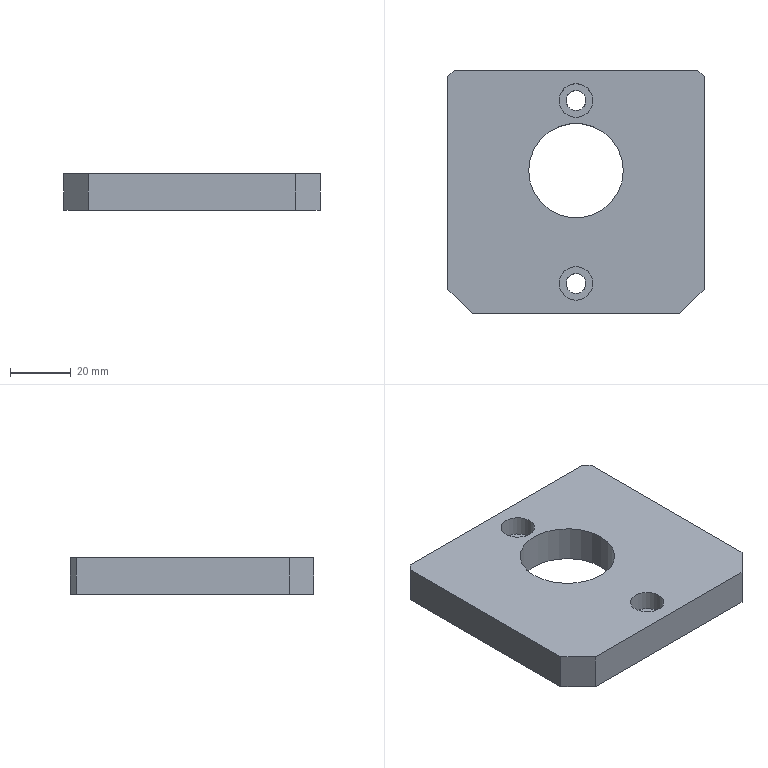Part | STEP file | P011002NM01-000 | 1 solid | 17 faces | box 84 x 80 x 12 mm | volume 69166 mm3 | plane 12 | cylinder 5 | commonest cylinder face diameters 6.5 x2 11 x2 31 x1
STEP:
#1=CARTESIAN_POINT('',(0.,0.,0.));
#2=DIRECTION('',(0.,0.,1.));
#3=DIRECTION('',(1.,0.,0.));
#4=AXIS2_PLACEMENT_3D('',#1,#2,#3);
#5=CARTESIAN_POINT('',(-104.,245.,9.));
#6=VERTEX_POINT('',#5);
#7=CARTESIAN_POINT('',(-172.,245.,9.));
#8=VERTEX_POINT('',#7);
#9=CARTESIAN_POINT('',(-140.,245.,9.));
#10=DIRECTION('',(-1.,0.,0.));
#11=VECTOR('',#10,1.);
#12=LINE('',#9,#11);
#13=CARTESIAN_POINT('',(-140.,245.,6.));
#14=DIRECTION('',(0.,-1.,0.));
#15=DIRECTION('',(0.,0.,-1.));
#16=AXIS2_PLACEMENT_3D('',#13,#14,#15);
#17=PLANE('',#16);
#18=CARTESIAN_POINT('',(-3.,0.));
#19=DIRECTION('',(0.,-1.));
#20=VECTOR('',#19,1.);
#21=LINE('',#18,#20);
#22=(GEOMETRIC_REPRESENTATION_CONTEXT(2)PARAMETRIC_REPRESENTATION_CONTEXT()REPRESENTATION_CONTEXT('',''));
#23=DEFINITIONAL_REPRESENTATION('',(#21),#22);
#24=PCURVE('',#17,#23);
#25=CARTESIAN_POINT('',(178.,-325.,9.));
#26=DIRECTION('',(0.,0.,1.));
#27=DIRECTION('',(1.,0.,0.));
#28=AXIS2_PLACEMENT_3D('',#25,#26,#27);
#29=PLANE('',#28);
#30=CARTESIAN_POINT('',(-318.,570.));
#31=DIRECTION('',(-1.,0.));
#32=VECTOR('',#31,1.);
#33=LINE('',#30,#32);
#34=(GEOMETRIC_REPRESENTATION_CONTEXT(2)PARAMETRIC_REPRESENTATION_CONTEXT()REPRESENTATION_CONTEXT('',''));
#35=DEFINITIONAL_REPRESENTATION('',(#33),#34);
#36=PCURVE('',#29,#35);
#37=SURFACE_CURVE('',#12,(#24,#36),.PCURVE_S1.);
#38=EDGE_CURVE('',#6,#8,#37,.T.);
#39=ORIENTED_EDGE('',*,*,#38,.F.);
#40=CARTESIAN_POINT('',(-104.,245.,21.));
#41=VERTEX_POINT('',#40);
#42=CARTESIAN_POINT('',(-104.,245.,6.));
#43=DIRECTION('',(0.,0.,1.));
#44=VECTOR('',#43,1.);
#45=LINE('',#42,#44);
#46=CARTESIAN_POINT('',(0.,36.));
#47=DIRECTION('',(-1.,0.));
#48=VECTOR('',#47,1.);
#49=LINE('',#46,#48);
#50=(GEOMETRIC_REPRESENTATION_CONTEXT(2)PARAMETRIC_REPRESENTATION_CONTEXT()REPRESENTATION_CONTEXT('',''));
#51=DEFINITIONAL_REPRESENTATION('',(#49),#50);
#52=PCURVE('',#17,#51);
#53=CARTESIAN_POINT('',(-96.,253.,6.));
#54=DIRECTION('',(-0.7071,0.7071,0.));
#55=DIRECTION('',(-0.7071,-0.7071,0.));
#56=AXIS2_PLACEMENT_3D('',#53,#54,#55);
#57=PLANE('',#56);
#58=CARTESIAN_POINT('',(11.314,0.));
#59=DIRECTION('',(0.,1.));
#60=VECTOR('',#59,1.);
#61=LINE('',#58,#60);
#62=(GEOMETRIC_REPRESENTATION_CONTEXT(2)PARAMETRIC_REPRESENTATION_CONTEXT()REPRESENTATION_CONTEXT('',''));
#63=DEFINITIONAL_REPRESENTATION('',(#61),#62);
#64=PCURVE('',#57,#63);
#65=SURFACE_CURVE('',#45,(#52,#64),.PCURVE_S1.);
#66=EDGE_CURVE('',#6,#41,#65,.T.);
#67=ORIENTED_EDGE('',*,*,#66,.T.);
#68=CARTESIAN_POINT('',(-172.,245.,21.));
#69=VERTEX_POINT('',#68);
#70=CARTESIAN_POINT('',(-140.,245.,21.));
#71=DIRECTION('',(-1.,0.,0.));
#72=VECTOR('',#71,1.);
#73=LINE('',#70,#72);
#74=CARTESIAN_POINT('',(-15.,0.));
#75=DIRECTION('',(0.,-1.));
#76=VECTOR('',#75,1.);
#77=LINE('',#74,#76);
#78=(GEOMETRIC_REPRESENTATION_CONTEXT(2)PARAMETRIC_REPRESENTATION_CONTEXT()REPRESENTATION_CONTEXT('',''));
#79=DEFINITIONAL_REPRESENTATION('',(#77),#78);
#80=PCURVE('',#17,#79);
#81=CARTESIAN_POINT('',(-130.,252.5,21.));
#82=DIRECTION('',(0.,0.,1.));
#83=DIRECTION('',(1.,0.,0.));
#84=AXIS2_PLACEMENT_3D('',#81,#82,#83);
#85=PLANE('',#84);
#86=CARTESIAN_POINT('',(-10.,-7.5));
#87=DIRECTION('',(-1.,0.));
#88=VECTOR('',#87,1.);
#89=LINE('',#86,#88);
#90=(GEOMETRIC_REPRESENTATION_CONTEXT(2)PARAMETRIC_REPRESENTATION_CONTEXT()REPRESENTATION_CONTEXT('',''));
#91=DEFINITIONAL_REPRESENTATION('',(#89),#90);
#92=PCURVE('',#85,#91);
#93=SURFACE_CURVE('',#73,(#80,#92),.PCURVE_S1.);
#94=EDGE_CURVE('',#41,#69,#93,.T.);
#95=ORIENTED_EDGE('',*,*,#94,.T.);
#96=CARTESIAN_POINT('',(-172.,245.,6.));
#97=DIRECTION('',(0.,0.,-1.));
#98=VECTOR('',#97,1.);
#99=LINE('',#96,#98);
#100=CARTESIAN_POINT('',(0.,-32.));
#101=DIRECTION('',(1.,0.));
#102=VECTOR('',#101,1.);
#103=LINE('',#100,#102);
#104=(GEOMETRIC_REPRESENTATION_CONTEXT(2)PARAMETRIC_REPRESENTATION_CONTEXT()REPRESENTATION_CONTEXT('',''));
#105=DEFINITIONAL_REPRESENTATION('',(#103),#104);
#106=PCURVE('',#17,#105);
#107=CARTESIAN_POINT('',(-172.,245.,6.));
#108=DIRECTION('',(0.7071,0.7071,0.));
#109=DIRECTION('',(-0.7071,0.7071,0.));
#110=AXIS2_PLACEMENT_3D('',#107,#108,#109);
#111=PLANE('',#110);
#112=CARTESIAN_POINT('',(0.,0.));
#113=DIRECTION('',(0.,-1.));
#114=VECTOR('',#113,1.);
#115=LINE('',#112,#114);
#116=(GEOMETRIC_REPRESENTATION_CONTEXT(2)PARAMETRIC_REPRESENTATION_CONTEXT()REPRESENTATION_CONTEXT('',''));
#117=DEFINITIONAL_REPRESENTATION('',(#115),#116);
#118=PCURVE('',#111,#117);
#119=SURFACE_CURVE('',#99,(#106,#118),.PCURVE_S1.);
#120=EDGE_CURVE('',#69,#8,#119,.T.);
#121=ORIENTED_EDGE('',*,*,#120,.T.);
#122=EDGE_LOOP('',(#39,#67,#95,#121));
#123=FACE_BOUND('',#122,.T.);
#124=ADVANCED_FACE('',(#123),#17,.T.);
#125=CARTESIAN_POINT('',(-96.,323.,9.));
#126=VERTEX_POINT('',#125);
#127=CARTESIAN_POINT('',(-96.,253.,9.));
#128=VERTEX_POINT('',#127);
#129=CARTESIAN_POINT('',(-96.,285.,9.));
#130=DIRECTION('',(0.,-1.,0.));
#131=VECTOR('',#130,1.);
#132=LINE('',#129,#131);
#133=CARTESIAN_POINT('',(-96.,285.,6.));
#134=DIRECTION('',(1.,0.,0.));
#135=DIRECTION('',(0.,0.,-1.));
#136=AXIS2_PLACEMENT_3D('',#133,#134,#135);
#137=PLANE('',#136);
#138=CARTESIAN_POINT('',(-3.,0.));
#139=DIRECTION('',(0.,-1.));
#140=VECTOR('',#139,1.);
#141=LINE('',#138,#140);
#142=(GEOMETRIC_REPRESENTATION_CONTEXT(2)PARAMETRIC_REPRESENTATION_CONTEXT()REPRESENTATION_CONTEXT('',''));
#143=DEFINITIONAL_REPRESENTATION('',(#141),#142);
#144=PCURVE('',#137,#143);
#145=CARTESIAN_POINT('',(-274.,610.));
#146=DIRECTION('',(0.,-1.));
#147=VECTOR('',#146,1.);
#148=LINE('',#145,#147);
#149=(GEOMETRIC_REPRESENTATION_CONTEXT(2)PARAMETRIC_REPRESENTATION_CONTEXT()REPRESENTATION_CONTEXT('',''));
#150=DEFINITIONAL_REPRESENTATION('',(#148),#149);
#151=PCURVE('',#29,#150);
#152=SURFACE_CURVE('',#132,(#144,#151),.PCURVE_S1.);
#153=EDGE_CURVE('',#126,#128,#152,.T.);
#154=ORIENTED_EDGE('',*,*,#153,.F.);
#155=CARTESIAN_POINT('',(-96.,323.,21.));
#156=VERTEX_POINT('',#155);
#157=CARTESIAN_POINT('',(-96.,323.,6.));
#158=DIRECTION('',(0.,0.,1.));
#159=VECTOR('',#158,1.);
#160=LINE('',#157,#159);
#161=CARTESIAN_POINT('',(0.,38.));
#162=DIRECTION('',(-1.,0.));
#163=VECTOR('',#162,1.);
#164=LINE('',#161,#163);
#165=(GEOMETRIC_REPRESENTATION_CONTEXT(2)PARAMETRIC_REPRESENTATION_CONTEXT()REPRESENTATION_CONTEXT('',''));
#166=DEFINITIONAL_REPRESENTATION('',(#164),#165);
#167=PCURVE('',#137,#166);
#168=CARTESIAN_POINT('',(-98.,325.,260.));
#169=DIRECTION('',(-0.7071,-0.7071,0.));
#170=DIRECTION('',(0.7071,-0.7071,0.));
#171=AXIS2_PLACEMENT_3D('',#168,#169,#170);
#172=PLANE('',#171);
#173=CARTESIAN_POINT('',(2.828,-254.));
#174=DIRECTION('',(0.,1.));
#175=VECTOR('',#174,1.);
#176=LINE('',#173,#175);
#177=(GEOMETRIC_REPRESENTATION_CONTEXT(2)PARAMETRIC_REPRESENTATION_CONTEXT()REPRESENTATION_CONTEXT('',''));
#178=DEFINITIONAL_REPRESENTATION('',(#176),#177);
#179=PCURVE('',#172,#178);
#180=SURFACE_CURVE('',#160,(#167,#179),.PCURVE_S1.);
#181=EDGE_CURVE('',#126,#156,#180,.T.);
#182=ORIENTED_EDGE('',*,*,#181,.T.);
#183=CARTESIAN_POINT('',(-96.,253.,21.));
#184=VERTEX_POINT('',#183);
#185=CARTESIAN_POINT('',(-96.,285.,21.));
#186=DIRECTION('',(0.,-1.,0.));
#187=VECTOR('',#186,1.);
#188=LINE('',#185,#187);
#189=CARTESIAN_POINT('',(-15.,0.));
#190=DIRECTION('',(0.,-1.));
#191=VECTOR('',#190,1.);
#192=LINE('',#189,#191);
#193=(GEOMETRIC_REPRESENTATION_CONTEXT(2)PARAMETRIC_REPRESENTATION_CONTEXT()REPRESENTATION_CONTEXT('',''));
#194=DEFINITIONAL_REPRESENTATION('',(#192),#193);
#195=PCURVE('',#137,#194);
#196=CARTESIAN_POINT('',(34.,32.5));
#197=DIRECTION('',(0.,-1.));
#198=VECTOR('',#197,1.);
#199=LINE('',#196,#198);
#200=(GEOMETRIC_REPRESENTATION_CONTEXT(2)PARAMETRIC_REPRESENTATION_CONTEXT()REPRESENTATION_CONTEXT('',''));
#201=DEFINITIONAL_REPRESENTATION('',(#199),#200);
#202=PCURVE('',#85,#201);
#203=SURFACE_CURVE('',#188,(#195,#202),.PCURVE_S1.);
#204=EDGE_CURVE('',#156,#184,#203,.T.);
#205=ORIENTED_EDGE('',*,*,#204,.T.);
#206=CARTESIAN_POINT('',(-96.,253.,6.));
#207=DIRECTION('',(0.,0.,-1.));
#208=VECTOR('',#207,1.);
#209=LINE('',#206,#208);
#210=CARTESIAN_POINT('',(0.,-32.));
#211=DIRECTION('',(1.,0.));
#212=VECTOR('',#211,1.);
#213=LINE('',#210,#212);
#214=(GEOMETRIC_REPRESENTATION_CONTEXT(2)PARAMETRIC_REPRESENTATION_CONTEXT()REPRESENTATION_CONTEXT('',''));
#215=DEFINITIONAL_REPRESENTATION('',(#213),#214);
#216=PCURVE('',#137,#215);
#217=CARTESIAN_POINT('',(0.,0.));
#218=DIRECTION('',(0.,-1.));
#219=VECTOR('',#218,1.);
#220=LINE('',#217,#219);
#221=(GEOMETRIC_REPRESENTATION_CONTEXT(2)PARAMETRIC_REPRESENTATION_CONTEXT()REPRESENTATION_CONTEXT('',''));
#222=DEFINITIONAL_REPRESENTATION('',(#220),#221);
#223=PCURVE('',#57,#222);
#224=SURFACE_CURVE('',#209,(#216,#223),.PCURVE_S1.);
#225=EDGE_CURVE('',#184,#128,#224,.T.);
#226=ORIENTED_EDGE('',*,*,#225,.T.);
#227=EDGE_LOOP('',(#154,#182,#205,#226));
#228=FACE_BOUND('',#227,.T.);
#229=ADVANCED_FACE('',(#228),#137,.T.);
#230=CARTESIAN_POINT('',(-178.,325.,9.));
#231=VERTEX_POINT('',#230);
#232=CARTESIAN_POINT('',(-98.,325.,9.));
#233=VERTEX_POINT('',#232);
#234=CARTESIAN_POINT('',(-325.,325.,9.));
#235=DIRECTION('',(1.,0.,0.));
#236=VECTOR('',#235,1.);
#237=LINE('',#234,#236);
#238=CARTESIAN_POINT('',(-325.,325.,260.));
#239=DIRECTION('',(0.,1.,0.));
#240=DIRECTION('',(0.,0.,1.));
#241=AXIS2_PLACEMENT_3D('',#238,#239,#240);
#242=PLANE('',#241);
#243=CARTESIAN_POINT('',(-251.,0.));
#244=DIRECTION('',(0.,1.));
#245=VECTOR('',#244,1.);
#246=LINE('',#243,#245);
#247=(GEOMETRIC_REPRESENTATION_CONTEXT(2)PARAMETRIC_REPRESENTATION_CONTEXT()REPRESENTATION_CONTEXT('',''));
#248=DEFINITIONAL_REPRESENTATION('',(#246),#247);
#249=PCURVE('',#242,#248);
#250=CARTESIAN_POINT('',(-503.,650.));
#251=DIRECTION('',(1.,0.));
#252=VECTOR('',#251,1.);
#253=LINE('',#250,#252);
#254=(GEOMETRIC_REPRESENTATION_CONTEXT(2)PARAMETRIC_REPRESENTATION_CONTEXT()REPRESENTATION_CONTEXT('',''));
#255=DEFINITIONAL_REPRESENTATION('',(#253),#254);
#256=PCURVE('',#29,#255);
#257=SURFACE_CURVE('',#237,(#249,#256),.PCURVE_S1.);
#258=EDGE_CURVE('',#231,#233,#257,.T.);
#259=ORIENTED_EDGE('',*,*,#258,.F.);
#260=CARTESIAN_POINT('',(-178.,325.,21.));
#261=VERTEX_POINT('',#260);
#262=CARTESIAN_POINT('',(-178.,325.,260.));
#263=DIRECTION('',(0.,0.,1.));
#264=VECTOR('',#263,1.);
#265=LINE('',#262,#264);
#266=CARTESIAN_POINT('',(0.,147.));
#267=DIRECTION('',(1.,0.));
#268=VECTOR('',#267,1.);
#269=LINE('',#266,#268);
#270=(GEOMETRIC_REPRESENTATION_CONTEXT(2)PARAMETRIC_REPRESENTATION_CONTEXT()REPRESENTATION_CONTEXT('',''));
#271=DEFINITIONAL_REPRESENTATION('',(#269),#270);
#272=PCURVE('',#242,#271);
#273=CARTESIAN_POINT('',(-180.,323.,6.));
#274=DIRECTION('',(0.7071,-0.7071,0.));
#275=DIRECTION('',(0.7071,0.7071,0.));
#276=AXIS2_PLACEMENT_3D('',#273,#274,#275);
#277=PLANE('',#276);
#278=CARTESIAN_POINT('',(2.828,254.));
#279=DIRECTION('',(0.,1.));
#280=VECTOR('',#279,1.);
#281=LINE('',#278,#280);
#282=(GEOMETRIC_REPRESENTATION_CONTEXT(2)PARAMETRIC_REPRESENTATION_CONTEXT()REPRESENTATION_CONTEXT('',''));
#283=DEFINITIONAL_REPRESENTATION('',(#281),#282);
#284=PCURVE('',#277,#283);
#285=SURFACE_CURVE('',#265,(#272,#284),.PCURVE_S1.);
#286=EDGE_CURVE('',#231,#261,#285,.T.);
#287=ORIENTED_EDGE('',*,*,#286,.T.);
#288=CARTESIAN_POINT('',(-98.,325.,21.));
#289=VERTEX_POINT('',#288);
#290=CARTESIAN_POINT('',(-325.,325.,21.));
#291=DIRECTION('',(1.,0.,0.));
#292=VECTOR('',#291,1.);
#293=LINE('',#290,#292);
#294=CARTESIAN_POINT('',(-239.,0.));
#295=DIRECTION('',(0.,1.));
#296=VECTOR('',#295,1.);
#297=LINE('',#294,#296);
#298=(GEOMETRIC_REPRESENTATION_CONTEXT(2)PARAMETRIC_REPRESENTATION_CONTEXT()REPRESENTATION_CONTEXT('',''));
#299=DEFINITIONAL_REPRESENTATION('',(#297),#298);
#300=PCURVE('',#242,#299);
#301=CARTESIAN_POINT('',(-195.,72.5));
#302=DIRECTION('',(1.,0.));
#303=VECTOR('',#302,1.);
#304=LINE('',#301,#303);
#305=(GEOMETRIC_REPRESENTATION_CONTEXT(2)PARAMETRIC_REPRESENTATION_CONTEXT()REPRESENTATION_CONTEXT('',''));
#306=DEFINITIONAL_REPRESENTATION('',(#304),#305);
#307=PCURVE('',#85,#306);
#308=SURFACE_CURVE('',#293,(#300,#307),.PCURVE_S1.);
#309=EDGE_CURVE('',#261,#289,#308,.T.);
#310=ORIENTED_EDGE('',*,*,#309,.T.);
#311=CARTESIAN_POINT('',(-98.,325.,260.));
#312=DIRECTION('',(0.,0.,-1.));
#313=VECTOR('',#312,1.);
#314=LINE('',#311,#313);
#315=CARTESIAN_POINT('',(0.,227.));
#316=DIRECTION('',(-1.,0.));
#317=VECTOR('',#316,1.);
#318=LINE('',#315,#317);
#319=(GEOMETRIC_REPRESENTATION_CONTEXT(2)PARAMETRIC_REPRESENTATION_CONTEXT()REPRESENTATION_CONTEXT('',''));
#320=DEFINITIONAL_REPRESENTATION('',(#318),#319);
#321=PCURVE('',#242,#320);
#322=CARTESIAN_POINT('',(0.,0.));
#323=DIRECTION('',(0.,-1.));
#324=VECTOR('',#323,1.);
#325=LINE('',#322,#324);
#326=(GEOMETRIC_REPRESENTATION_CONTEXT(2)PARAMETRIC_REPRESENTATION_CONTEXT()REPRESENTATION_CONTEXT('',''));
#327=DEFINITIONAL_REPRESENTATION('',(#325),#326);
#328=PCURVE('',#172,#327);
#329=SURFACE_CURVE('',#314,(#321,#328),.PCURVE_S1.);
#330=EDGE_CURVE('',#289,#233,#329,.T.);
#331=ORIENTED_EDGE('',*,*,#330,.T.);
#332=EDGE_LOOP('',(#259,#287,#310,#331));
#333=FACE_BOUND('',#332,.T.);
#334=ADVANCED_FACE('',(#333),#242,.T.);
#335=CARTESIAN_POINT('',(-138.,249.5,21.));
#336=VERTEX_POINT('',#335);
#337=CARTESIAN_POINT('',(-138.,255.,21.));
#338=DIRECTION('',(0.,0.,1.));
#339=DIRECTION('',(0.,-1.,0.));
#340=AXIS2_PLACEMENT_3D('',#337,#338,#339);
#341=CIRCLE('',#340,5.5);
#342=CARTESIAN_POINT('',(-8.,2.5));
#343=DIRECTION('',(0.,-1.));
#344=AXIS2_PLACEMENT_2D('',#342,#343);
#345=CIRCLE('',#344,5.5);
#346=(GEOMETRIC_REPRESENTATION_CONTEXT(2)PARAMETRIC_REPRESENTATION_CONTEXT()REPRESENTATION_CONTEXT('',''));
#347=DEFINITIONAL_REPRESENTATION('',(#345),#346);
#348=PCURVE('',#85,#347);
#349=CARTESIAN_POINT('',(-138.,255.,22.));
#350=DIRECTION('',(0.,0.,1.));
#351=DIRECTION('',(0.,-1.,0.));
#352=AXIS2_PLACEMENT_3D('',#349,#350,#351);
#353=CYLINDRICAL_SURFACE('',#352,5.5);
#354=CARTESIAN_POINT('',(0.,-1.));
#355=DIRECTION('',(1.,0.));
#356=VECTOR('',#355,1.);
#357=LINE('',#354,#356);
#358=(GEOMETRIC_REPRESENTATION_CONTEXT(2)PARAMETRIC_REPRESENTATION_CONTEXT()REPRESENTATION_CONTEXT('',''));
#359=DEFINITIONAL_REPRESENTATION('',(#357),#358);
#360=PCURVE('',#353,#359);
#361=SURFACE_CURVE('',#341,(#348,#360),.PCURVE_S1.);
#362=EDGE_CURVE('',#336,#336,#361,.T.);
#363=ORIENTED_EDGE('',*,*,#362,.F.);
#364=EDGE_LOOP('',(#363));
#365=FACE_BOUND('',#364,.T.);
#366=CARTESIAN_POINT('',(-138.,309.5,21.));
#367=VERTEX_POINT('',#366);
#368=CARTESIAN_POINT('',(-138.,315.,21.));
#369=DIRECTION('',(0.,0.,1.));
#370=DIRECTION('',(0.,-1.,0.));
#371=AXIS2_PLACEMENT_3D('',#368,#369,#370);
#372=CIRCLE('',#371,5.5);
#373=CARTESIAN_POINT('',(-8.,62.5));
#374=DIRECTION('',(0.,-1.));
#375=AXIS2_PLACEMENT_2D('',#373,#374);
#376=CIRCLE('',#375,5.5);
#377=(GEOMETRIC_REPRESENTATION_CONTEXT(2)PARAMETRIC_REPRESENTATION_CONTEXT()REPRESENTATION_CONTEXT('',''));
#378=DEFINITIONAL_REPRESENTATION('',(#376),#377);
#379=PCURVE('',#85,#378);
#380=CARTESIAN_POINT('',(-138.,315.,22.));
#381=DIRECTION('',(0.,0.,1.));
#382=DIRECTION('',(0.,-1.,0.));
#383=AXIS2_PLACEMENT_3D('',#380,#381,#382);
#384=CYLINDRICAL_SURFACE('',#383,5.5);
#385=CARTESIAN_POINT('',(0.,-1.));
#386=DIRECTION('',(1.,0.));
#387=VECTOR('',#386,1.);
#388=LINE('',#385,#387);
#389=(GEOMETRIC_REPRESENTATION_CONTEXT(2)PARAMETRIC_REPRESENTATION_CONTEXT()REPRESENTATION_CONTEXT('',''));
#390=DEFINITIONAL_REPRESENTATION('',(#388),#389);
#391=PCURVE('',#384,#390);
#392=SURFACE_CURVE('',#372,(#379,#391),.PCURVE_S1.);
#393=EDGE_CURVE('',#367,#367,#392,.T.);
#394=ORIENTED_EDGE('',*,*,#393,.F.);
#395=EDGE_LOOP('',(#394));
#396=FACE_BOUND('',#395,.T.);
#397=CARTESIAN_POINT('',(-122.5,292.,21.));
#398=VERTEX_POINT('',#397);
#399=CARTESIAN_POINT('',(-138.,292.,21.));
#400=DIRECTION('',(0.,0.,1.));
#401=DIRECTION('',(1.,0.,0.));
#402=AXIS2_PLACEMENT_3D('',#399,#400,#401);
#403=CIRCLE('',#402,15.5);
#404=CARTESIAN_POINT('',(-8.,39.5));
#405=DIRECTION('',(1.,0.));
#406=AXIS2_PLACEMENT_2D('',#404,#405);
#407=CIRCLE('',#406,15.5);
#408=(GEOMETRIC_REPRESENTATION_CONTEXT(2)PARAMETRIC_REPRESENTATION_CONTEXT()REPRESENTATION_CONTEXT('',''));
#409=DEFINITIONAL_REPRESENTATION('',(#407),#408);
#410=PCURVE('',#85,#409);
#411=CARTESIAN_POINT('',(-138.,292.,539.));
#412=DIRECTION('',(0.,0.,-1.));
#413=DIRECTION('',(1.,0.,0.));
#414=AXIS2_PLACEMENT_3D('',#411,#412,#413);
#415=CYLINDRICAL_SURFACE('',#414,15.5);
#416=CARTESIAN_POINT('',(6.283,518.));
#417=DIRECTION('',(-1.,0.));
#418=VECTOR('',#417,1.);
#419=LINE('',#416,#418);
#420=(GEOMETRIC_REPRESENTATION_CONTEXT(2)PARAMETRIC_REPRESENTATION_CONTEXT()REPRESENTATION_CONTEXT('',''));
#421=DEFINITIONAL_REPRESENTATION('',(#419),#420);
#422=PCURVE('',#415,#421);
#423=SURFACE_CURVE('',#403,(#410,#422),.PCURVE_S1.);
#424=EDGE_CURVE('',#398,#398,#423,.T.);
#425=ORIENTED_EDGE('',*,*,#424,.F.);
#426=EDGE_LOOP('',(#425));
#427=FACE_BOUND('',#426,.T.);
#428=ORIENTED_EDGE('',*,*,#204,.F.);
#429=CARTESIAN_POINT('',(-75.75,302.75,21.));
#430=DIRECTION('',(-0.7071,0.7071,0.));
#431=VECTOR('',#430,1.);
#432=LINE('',#429,#431);
#433=CARTESIAN_POINT('',(54.25,50.25));
#434=DIRECTION('',(-0.7071,0.7071));
#435=VECTOR('',#434,1.);
#436=LINE('',#433,#435);
#437=(GEOMETRIC_REPRESENTATION_CONTEXT(2)PARAMETRIC_REPRESENTATION_CONTEXT()REPRESENTATION_CONTEXT('',''));
#438=DEFINITIONAL_REPRESENTATION('',(#436),#437);
#439=PCURVE('',#85,#438);
#440=CARTESIAN_POINT('',(31.466,-239.));
#441=DIRECTION('',(-1.,0.));
#442=VECTOR('',#441,1.);
#443=LINE('',#440,#442);
#444=(GEOMETRIC_REPRESENTATION_CONTEXT(2)PARAMETRIC_REPRESENTATION_CONTEXT()REPRESENTATION_CONTEXT('',''));
#445=DEFINITIONAL_REPRESENTATION('',(#443),#444);
#446=PCURVE('',#172,#445);
#447=SURFACE_CURVE('',#432,(#439,#446),.PCURVE_S1.);
#448=EDGE_CURVE('',#156,#289,#447,.T.);
#449=ORIENTED_EDGE('',*,*,#448,.T.);
#450=ORIENTED_EDGE('',*,*,#309,.F.);
#451=CARTESIAN_POINT('',(-180.,323.,21.));
#452=VERTEX_POINT('',#451);
#453=CARTESIAN_POINT('',(-190.25,312.75,21.));
#454=DIRECTION('',(-0.7071,-0.7071,0.));
#455=VECTOR('',#454,1.);
#456=LINE('',#453,#455);
#457=CARTESIAN_POINT('',(-60.25,60.25));
#458=DIRECTION('',(-0.7071,-0.7071));
#459=VECTOR('',#458,1.);
#460=LINE('',#457,#459);
#461=(GEOMETRIC_REPRESENTATION_CONTEXT(2)PARAMETRIC_REPRESENTATION_CONTEXT()REPRESENTATION_CONTEXT('',''));
#462=DEFINITIONAL_REPRESENTATION('',(#460),#461);
#463=PCURVE('',#85,#462);
#464=CARTESIAN_POINT('',(-14.496,15.));
#465=DIRECTION('',(-1.,0.));
#466=VECTOR('',#465,1.);
#467=LINE('',#464,#466);
#468=(GEOMETRIC_REPRESENTATION_CONTEXT(2)PARAMETRIC_REPRESENTATION_CONTEXT()REPRESENTATION_CONTEXT('',''));
#469=DEFINITIONAL_REPRESENTATION('',(#467),#468);
#470=PCURVE('',#277,#469);
#471=SURFACE_CURVE('',#456,(#463,#470),.PCURVE_S1.);
#472=EDGE_CURVE('',#261,#452,#471,.T.);
#473=ORIENTED_EDGE('',*,*,#472,.T.);
#474=CARTESIAN_POINT('',(-180.,253.,21.));
#475=VERTEX_POINT('',#474);
#476=CARTESIAN_POINT('',(-180.,285.,21.));
#477=DIRECTION('',(0.,1.,0.));
#478=VECTOR('',#477,1.);
#479=LINE('',#476,#478);
#480=CARTESIAN_POINT('',(-50.,32.5));
#481=DIRECTION('',(0.,1.));
#482=VECTOR('',#481,1.);
#483=LINE('',#480,#482);
#484=(GEOMETRIC_REPRESENTATION_CONTEXT(2)PARAMETRIC_REPRESENTATION_CONTEXT()REPRESENTATION_CONTEXT('',''));
#485=DEFINITIONAL_REPRESENTATION('',(#483),#484);
#486=PCURVE('',#85,#485);
#487=CARTESIAN_POINT('',(-180.,285.,6.));
#488=DIRECTION('',(-1.,0.,0.));
#489=DIRECTION('',(0.,0.,1.));
#490=AXIS2_PLACEMENT_3D('',#487,#488,#489);
#491=PLANE('',#490);
#492=CARTESIAN_POINT('',(15.,0.));
#493=DIRECTION('',(0.,1.));
#494=VECTOR('',#493,1.);
#495=LINE('',#492,#494);
#496=(GEOMETRIC_REPRESENTATION_CONTEXT(2)PARAMETRIC_REPRESENTATION_CONTEXT()REPRESENTATION_CONTEXT('',''));
#497=DEFINITIONAL_REPRESENTATION('',(#495),#496);
#498=PCURVE('',#491,#497);
#499=SURFACE_CURVE('',#479,(#486,#498),.PCURVE_S1.);
#500=EDGE_CURVE('',#475,#452,#499,.T.);
#501=ORIENTED_EDGE('',*,*,#500,.F.);
#502=CARTESIAN_POINT('',(-154.75,227.75,21.));
#503=DIRECTION('',(0.7071,-0.7071,0.));
#504=VECTOR('',#503,1.);
#505=LINE('',#502,#504);
#506=CARTESIAN_POINT('',(-24.75,-24.75));
#507=DIRECTION('',(0.7071,-0.7071));
#508=VECTOR('',#507,1.);
#509=LINE('',#506,#508);
#510=(GEOMETRIC_REPRESENTATION_CONTEXT(2)PARAMETRIC_REPRESENTATION_CONTEXT()REPRESENTATION_CONTEXT('',''));
#511=DEFINITIONAL_REPRESENTATION('',(#509),#510);
#512=PCURVE('',#85,#511);
#513=CARTESIAN_POINT('',(-24.395,15.));
#514=DIRECTION('',(-1.,0.));
#515=VECTOR('',#514,1.);
#516=LINE('',#513,#515);
#517=(GEOMETRIC_REPRESENTATION_CONTEXT(2)PARAMETRIC_REPRESENTATION_CONTEXT()REPRESENTATION_CONTEXT('',''));
#518=DEFINITIONAL_REPRESENTATION('',(#516),#517);
#519=PCURVE('',#111,#518);
#520=SURFACE_CURVE('',#505,(#512,#519),.PCURVE_S1.);
#521=EDGE_CURVE('',#475,#69,#520,.T.);
#522=ORIENTED_EDGE('',*,*,#521,.T.);
#523=ORIENTED_EDGE('',*,*,#94,.F.);
#524=CARTESIAN_POINT('',(-111.25,237.75,21.));
#525=DIRECTION('',(0.7071,0.7071,0.));
#526=VECTOR('',#525,1.);
#527=LINE('',#524,#526);
#528=CARTESIAN_POINT('',(18.75,-14.75));
#529=DIRECTION('',(0.7071,0.7071));
#530=VECTOR('',#529,1.);
#531=LINE('',#528,#530);
#532=(GEOMETRIC_REPRESENTATION_CONTEXT(2)PARAMETRIC_REPRESENTATION_CONTEXT()REPRESENTATION_CONTEXT('',''));
#533=DEFINITIONAL_REPRESENTATION('',(#531),#532);
#534=PCURVE('',#85,#533);
#535=CARTESIAN_POINT('',(21.567,15.));
#536=DIRECTION('',(-1.,0.));
#537=VECTOR('',#536,1.);
#538=LINE('',#535,#537);
#539=(GEOMETRIC_REPRESENTATION_CONTEXT(2)PARAMETRIC_REPRESENTATION_CONTEXT()REPRESENTATION_CONTEXT('',''));
#540=DEFINITIONAL_REPRESENTATION('',(#538),#539);
#541=PCURVE('',#57,#540);
#542=SURFACE_CURVE('',#527,(#534,#541),.PCURVE_S1.);
#543=EDGE_CURVE('',#41,#184,#542,.T.);
#544=ORIENTED_EDGE('',*,*,#543,.T.);
#545=EDGE_LOOP('',(#428,#449,#450,#473,#501,#522,#523,#544));
#546=FACE_BOUND('',#545,.T.);
#547=ADVANCED_FACE('',(#365,#396,#427,#546),#85,.T.);
#548=CARTESIAN_POINT('',(-180.,253.,9.));
#549=VERTEX_POINT('',#548);
#550=CARTESIAN_POINT('',(-180.,323.,9.));
#551=VERTEX_POINT('',#550);
#552=CARTESIAN_POINT('',(-180.,285.,9.));
#553=DIRECTION('',(0.,1.,0.));
#554=VECTOR('',#553,1.);
#555=LINE('',#552,#554);
#556=CARTESIAN_POINT('',(3.,0.));
#557=DIRECTION('',(0.,1.));
#558=VECTOR('',#557,1.);
#559=LINE('',#556,#558);
#560=(GEOMETRIC_REPRESENTATION_CONTEXT(2)PARAMETRIC_REPRESENTATION_CONTEXT()REPRESENTATION_CONTEXT('',''));
#561=DEFINITIONAL_REPRESENTATION('',(#559),#560);
#562=PCURVE('',#491,#561);
#563=CARTESIAN_POINT('',(-358.,610.));
#564=DIRECTION('',(0.,1.));
#565=VECTOR('',#564,1.);
#566=LINE('',#563,#565);
#567=(GEOMETRIC_REPRESENTATION_CONTEXT(2)PARAMETRIC_REPRESENTATION_CONTEXT()REPRESENTATION_CONTEXT('',''));
#568=DEFINITIONAL_REPRESENTATION('',(#566),#567);
#569=PCURVE('',#29,#568);
#570=SURFACE_CURVE('',#555,(#562,#569),.PCURVE_S1.);
#571=EDGE_CURVE('',#549,#551,#570,.T.);
#572=ORIENTED_EDGE('',*,*,#571,.F.);
#573=CARTESIAN_POINT('',(-180.,253.,6.));
#574=DIRECTION('',(0.,0.,1.));
#575=VECTOR('',#574,1.);
#576=LINE('',#573,#575);
#577=CARTESIAN_POINT('',(0.,-32.));
#578=DIRECTION('',(1.,0.));
#579=VECTOR('',#578,1.);
#580=LINE('',#577,#579);
#581=(GEOMETRIC_REPRESENTATION_CONTEXT(2)PARAMETRIC_REPRESENTATION_CONTEXT()REPRESENTATION_CONTEXT('',''));
#582=DEFINITIONAL_REPRESENTATION('',(#580),#581);
#583=PCURVE('',#491,#582);
#584=CARTESIAN_POINT('',(11.314,0.));
#585=DIRECTION('',(0.,1.));
#586=VECTOR('',#585,1.);
#587=LINE('',#584,#586);
#588=(GEOMETRIC_REPRESENTATION_CONTEXT(2)PARAMETRIC_REPRESENTATION_CONTEXT()REPRESENTATION_CONTEXT('',''));
#589=DEFINITIONAL_REPRESENTATION('',(#587),#588);
#590=PCURVE('',#111,#589);
#591=SURFACE_CURVE('',#576,(#583,#590),.PCURVE_S1.);
#592=EDGE_CURVE('',#549,#475,#591,.T.);
#593=ORIENTED_EDGE('',*,*,#592,.T.);
#594=ORIENTED_EDGE('',*,*,#500,.T.);
#595=CARTESIAN_POINT('',(-180.,323.,6.));
#596=DIRECTION('',(0.,0.,-1.));
#597=VECTOR('',#596,1.);
#598=LINE('',#595,#597);
#599=CARTESIAN_POINT('',(0.,38.));
#600=DIRECTION('',(-1.,0.));
#601=VECTOR('',#600,1.);
#602=LINE('',#599,#601);
#603=(GEOMETRIC_REPRESENTATION_CONTEXT(2)PARAMETRIC_REPRESENTATION_CONTEXT()REPRESENTATION_CONTEXT('',''));
#604=DEFINITIONAL_REPRESENTATION('',(#602),#603);
#605=PCURVE('',#491,#604);
#606=CARTESIAN_POINT('',(0.,0.));
#607=DIRECTION('',(0.,-1.));
#608=VECTOR('',#607,1.);
#609=LINE('',#606,#608);
#610=(GEOMETRIC_REPRESENTATION_CONTEXT(2)PARAMETRIC_REPRESENTATION_CONTEXT()REPRESENTATION_CONTEXT('',''));
#611=DEFINITIONAL_REPRESENTATION('',(#609),#610);
#612=PCURVE('',#277,#611);
#613=SURFACE_CURVE('',#598,(#605,#612),.PCURVE_S1.);
#614=EDGE_CURVE('',#452,#551,#613,.T.);
#615=ORIENTED_EDGE('',*,*,#614,.T.);
#616=EDGE_LOOP('',(#572,#593,#594,#615));
#617=FACE_BOUND('',#616,.T.);
#618=ADVANCED_FACE('',(#617),#491,.T.);
#619=CARTESIAN_POINT('',(-96.,253.,9.));
#620=DIRECTION('',(-0.7071,-0.7071,0.));
#621=VECTOR('',#620,1.);
#622=LINE('',#619,#621);
#623=CARTESIAN_POINT('',(0.,3.));
#624=DIRECTION('',(1.,0.));
#625=VECTOR('',#624,1.);
#626=LINE('',#623,#625);
#627=(GEOMETRIC_REPRESENTATION_CONTEXT(2)PARAMETRIC_REPRESENTATION_CONTEXT()REPRESENTATION_CONTEXT('',''));
#628=DEFINITIONAL_REPRESENTATION('',(#626),#627);
#629=PCURVE('',#57,#628);
#630=CARTESIAN_POINT('',(-274.,578.));
#631=DIRECTION('',(-0.7071,-0.7071));
#632=VECTOR('',#631,1.);
#633=LINE('',#630,#632);
#634=(GEOMETRIC_REPRESENTATION_CONTEXT(2)PARAMETRIC_REPRESENTATION_CONTEXT()REPRESENTATION_CONTEXT('',''));
#635=DEFINITIONAL_REPRESENTATION('',(#633),#634);
#636=PCURVE('',#29,#635);
#637=SURFACE_CURVE('',#622,(#629,#636),.PCURVE_S1.);
#638=EDGE_CURVE('',#128,#6,#637,.T.);
#639=ORIENTED_EDGE('',*,*,#638,.F.);
#640=ORIENTED_EDGE('',*,*,#225,.F.);
#641=ORIENTED_EDGE('',*,*,#543,.F.);
#642=ORIENTED_EDGE('',*,*,#66,.F.);
#643=EDGE_LOOP('',(#639,#640,#641,#642));
#644=FACE_BOUND('',#643,.T.);
#645=ADVANCED_FACE('',(#644),#57,.F.);
#646=CARTESIAN_POINT('',(-172.,245.,9.));
#647=DIRECTION('',(-0.7071,0.7071,0.));
#648=VECTOR('',#647,1.);
#649=LINE('',#646,#648);
#650=CARTESIAN_POINT('',(0.,3.));
#651=DIRECTION('',(1.,0.));
#652=VECTOR('',#651,1.);
#653=LINE('',#650,#652);
#654=(GEOMETRIC_REPRESENTATION_CONTEXT(2)PARAMETRIC_REPRESENTATION_CONTEXT()REPRESENTATION_CONTEXT('',''));
#655=DEFINITIONAL_REPRESENTATION('',(#653),#654);
#656=PCURVE('',#111,#655);
#657=CARTESIAN_POINT('',(-350.,570.));
#658=DIRECTION('',(-0.7071,0.7071));
#659=VECTOR('',#658,1.);
#660=LINE('',#657,#659);
#661=(GEOMETRIC_REPRESENTATION_CONTEXT(2)PARAMETRIC_REPRESENTATION_CONTEXT()REPRESENTATION_CONTEXT('',''));
#662=DEFINITIONAL_REPRESENTATION('',(#660),#661);
#663=PCURVE('',#29,#662);
#664=SURFACE_CURVE('',#649,(#656,#663),.PCURVE_S1.);
#665=EDGE_CURVE('',#8,#549,#664,.T.);
#666=ORIENTED_EDGE('',*,*,#665,.F.);
#667=ORIENTED_EDGE('',*,*,#120,.F.);
#668=ORIENTED_EDGE('',*,*,#521,.F.);
#669=ORIENTED_EDGE('',*,*,#592,.F.);
#670=EDGE_LOOP('',(#666,#667,#668,#669));
#671=FACE_BOUND('',#670,.T.);
#672=ADVANCED_FACE('',(#671),#111,.F.);
#673=CARTESIAN_POINT('',(-98.,325.,9.));
#674=DIRECTION('',(0.7071,-0.7071,0.));
#675=VECTOR('',#674,1.);
#676=LINE('',#673,#675);
#677=CARTESIAN_POINT('',(0.,-251.));
#678=DIRECTION('',(1.,0.));
#679=VECTOR('',#678,1.);
#680=LINE('',#677,#679);
#681=(GEOMETRIC_REPRESENTATION_CONTEXT(2)PARAMETRIC_REPRESENTATION_CONTEXT()REPRESENTATION_CONTEXT('',''));
#682=DEFINITIONAL_REPRESENTATION('',(#680),#681);
#683=PCURVE('',#172,#682);
#684=CARTESIAN_POINT('',(-276.,650.));
#685=DIRECTION('',(0.7071,-0.7071));
#686=VECTOR('',#685,1.);
#687=LINE('',#684,#686);
#688=(GEOMETRIC_REPRESENTATION_CONTEXT(2)PARAMETRIC_REPRESENTATION_CONTEXT()REPRESENTATION_CONTEXT('',''));
#689=DEFINITIONAL_REPRESENTATION('',(#687),#688);
#690=PCURVE('',#29,#689);
#691=SURFACE_CURVE('',#676,(#683,#690),.PCURVE_S1.);
#692=EDGE_CURVE('',#233,#126,#691,.T.);
#693=ORIENTED_EDGE('',*,*,#692,.F.);
#694=ORIENTED_EDGE('',*,*,#330,.F.);
#695=ORIENTED_EDGE('',*,*,#448,.F.);
#696=ORIENTED_EDGE('',*,*,#181,.F.);
#697=EDGE_LOOP('',(#693,#694,#695,#696));
#698=FACE_BOUND('',#697,.T.);
#699=ADVANCED_FACE('',(#698),#172,.F.);
#700=CARTESIAN_POINT('',(-180.,323.,9.));
#701=DIRECTION('',(0.7071,0.7071,0.));
#702=VECTOR('',#701,1.);
#703=LINE('',#700,#702);
#704=CARTESIAN_POINT('',(0.,3.));
#705=DIRECTION('',(1.,0.));
#706=VECTOR('',#705,1.);
#707=LINE('',#704,#706);
#708=(GEOMETRIC_REPRESENTATION_CONTEXT(2)PARAMETRIC_REPRESENTATION_CONTEXT()REPRESENTATION_CONTEXT('',''));
#709=DEFINITIONAL_REPRESENTATION('',(#707),#708);
#710=PCURVE('',#277,#709);
#711=CARTESIAN_POINT('',(-358.,648.));
#712=DIRECTION('',(0.7071,0.7071));
#713=VECTOR('',#712,1.);
#714=LINE('',#711,#713);
#715=(GEOMETRIC_REPRESENTATION_CONTEXT(2)PARAMETRIC_REPRESENTATION_CONTEXT()REPRESENTATION_CONTEXT('',''));
#716=DEFINITIONAL_REPRESENTATION('',(#714),#715);
#717=PCURVE('',#29,#716);
#718=SURFACE_CURVE('',#703,(#710,#717),.PCURVE_S1.);
#719=EDGE_CURVE('',#551,#231,#718,.T.);
#720=ORIENTED_EDGE('',*,*,#719,.F.);
#721=ORIENTED_EDGE('',*,*,#614,.F.);
#722=ORIENTED_EDGE('',*,*,#472,.F.);
#723=ORIENTED_EDGE('',*,*,#286,.F.);
#724=EDGE_LOOP('',(#720,#721,#722,#723));
#725=FACE_BOUND('',#724,.T.);
#726=ADVANCED_FACE('',(#725),#277,.F.);
#727=CARTESIAN_POINT('',(-122.5,292.,9.));
#728=VERTEX_POINT('',#727);
#729=CARTESIAN_POINT('',(-138.,292.,9.));
#730=DIRECTION('',(0.,0.,-1.));
#731=DIRECTION('',(1.,0.,0.));
#732=AXIS2_PLACEMENT_3D('',#729,#730,#731);
#733=CIRCLE('',#732,15.5);
#734=CARTESIAN_POINT('',(0.,530.));
#735=DIRECTION('',(1.,0.));
#736=VECTOR('',#735,1.);
#737=LINE('',#734,#736);
#738=(GEOMETRIC_REPRESENTATION_CONTEXT(2)PARAMETRIC_REPRESENTATION_CONTEXT()REPRESENTATION_CONTEXT('',''));
#739=DEFINITIONAL_REPRESENTATION('',(#737),#738);
#740=PCURVE('',#415,#739);
#741=CARTESIAN_POINT('',(-300.5,617.));
#742=CARTESIAN_POINT('',(-300.5,590.153));
#743=CARTESIAN_POINT('',(-323.75,603.577));
#744=CARTESIAN_POINT('',(-347.,617.));
#745=CARTESIAN_POINT('',(-323.75,630.423));
#746=CARTESIAN_POINT('',(-300.5,643.847));
#747=CARTESIAN_POINT('',(-300.5,617.));
#748=(BOUNDED_CURVE()B_SPLINE_CURVE(2,(#741,#742,#743,#744,#745,#746,#747),.UNSPECIFIED.,.T.,.F.)B_SPLINE_CURVE_WITH_KNOTS((1,2,2,2,2,1),(-2.094,0.,2.094,4.189,6.283,8.378),.UNSPECIFIED.)CURVE()GEOMETRIC_REPRESENTATION_ITEM()RATIONAL_B_SPLINE_CURVE((1.,0.5,1.,0.5,1.,0.5,1.))REPRESENTATION_ITEM(''));
#749=(GEOMETRIC_REPRESENTATION_CONTEXT(2)PARAMETRIC_REPRESENTATION_CONTEXT()REPRESENTATION_CONTEXT('',''));
#750=DEFINITIONAL_REPRESENTATION('',(#748),#749);
#751=PCURVE('',#29,#750);
#752=SURFACE_CURVE('',#733,(#740,#751),.PCURVE_S1.);
#753=EDGE_CURVE('',#728,#728,#752,.T.);
#754=ORIENTED_EDGE('',*,*,#753,.F.);
#755=CARTESIAN_POINT('',(-122.5,292.,21.));
#756=CARTESIAN_POINT('',(-122.5,292.,9.));
#757=B_SPLINE_CURVE_WITH_KNOTS('',1,(#755,#756),.UNSPECIFIED.,.F.,.F.,(2,2),(518.,530.),.PIECEWISE_BEZIER_KNOTS.);
#758=CARTESIAN_POINT('',(0.,0.));
#759=DIRECTION('',(0.,1.));
#760=VECTOR('',#759,1.);
#761=LINE('',#758,#760);
#762=(GEOMETRIC_REPRESENTATION_CONTEXT(2)PARAMETRIC_REPRESENTATION_CONTEXT()REPRESENTATION_CONTEXT('',''));
#763=DEFINITIONAL_REPRESENTATION('',(#761),#762);
#764=PCURVE('',#415,#763);
#765=CARTESIAN_POINT('',(6.283,0.));
#766=DIRECTION('',(0.,1.));
#767=VECTOR('',#766,1.);
#768=LINE('',#765,#767);
#769=(GEOMETRIC_REPRESENTATION_CONTEXT(2)PARAMETRIC_REPRESENTATION_CONTEXT()REPRESENTATION_CONTEXT('',''));
#770=DEFINITIONAL_REPRESENTATION('',(#768),#769);
#771=PCURVE('',#415,#770);
#772=SEAM_CURVE('',#757,(#764,#771),.PCURVE_S1.);
#773=EDGE_CURVE('',#398,#728,#772,.T.);
#774=ORIENTED_EDGE('',*,*,#773,.F.);
#775=ORIENTED_EDGE('',*,*,#424,.F.);
#776=ORIENTED_EDGE('',*,*,#773,.T.);
#777=EDGE_LOOP('',(#754,#774,#775,#776));
#778=FACE_BOUND('',#777,.F.);
#779=ADVANCED_FACE('',(#778),#415,.F.);
#780=CARTESIAN_POINT('',(-134.75,255.,9.));
#781=VERTEX_POINT('',#780);
#782=CARTESIAN_POINT('',(-138.,251.75,9.));
#783=VERTEX_POINT('',#782);
#784=CARTESIAN_POINT('',(-138.,255.,9.));
#785=DIRECTION('',(0.,0.,1.));
#786=DIRECTION('',(1.,0.,0.));
#787=AXIS2_PLACEMENT_3D('',#784,#785,#786);
#788=CIRCLE('',#787,3.25);
#789=CARTESIAN_POINT('',(-316.,580.));
#790=DIRECTION('',(1.,0.));
#791=AXIS2_PLACEMENT_2D('',#789,#790);
#792=CIRCLE('',#791,3.25);
#793=(GEOMETRIC_REPRESENTATION_CONTEXT(2)PARAMETRIC_REPRESENTATION_CONTEXT()REPRESENTATION_CONTEXT('',''));
#794=DEFINITIONAL_REPRESENTATION('',(#792),#793);
#795=PCURVE('',#29,#794);
#796=CARTESIAN_POINT('',(-138.,255.,22.));
#797=DIRECTION('',(0.,0.,1.));
#798=DIRECTION('',(0.,-1.,0.));
#799=AXIS2_PLACEMENT_3D('',#796,#797,#798);
#800=CYLINDRICAL_SURFACE('',#799,3.25);
#801=CARTESIAN_POINT('',(1.571,-13.));
#802=DIRECTION('',(1.,0.));
#803=VECTOR('',#802,1.);
#804=LINE('',#801,#803);
#805=(GEOMETRIC_REPRESENTATION_CONTEXT(2)PARAMETRIC_REPRESENTATION_CONTEXT()REPRESENTATION_CONTEXT('',''));
#806=DEFINITIONAL_REPRESENTATION('',(#804),#805);
#807=PCURVE('',#800,#806);
#808=SURFACE_CURVE('',#788,(#795,#807),.PCURVE_S1.);
#809=EDGE_CURVE('',#781,#783,#808,.T.);
#810=ORIENTED_EDGE('',*,*,#809,.T.);
#811=CARTESIAN_POINT('',(-138.,255.,9.));
#812=DIRECTION('',(0.,0.,1.));
#813=DIRECTION('',(1.,0.,0.));
#814=AXIS2_PLACEMENT_3D('',#811,#812,#813);
#815=CIRCLE('',#814,3.25);
#816=CARTESIAN_POINT('',(-316.,580.));
#817=DIRECTION('',(1.,0.));
#818=AXIS2_PLACEMENT_2D('',#816,#817);
#819=CIRCLE('',#818,3.25);
#820=(GEOMETRIC_REPRESENTATION_CONTEXT(2)PARAMETRIC_REPRESENTATION_CONTEXT()REPRESENTATION_CONTEXT('',''));
#821=DEFINITIONAL_REPRESENTATION('',(#819),#820);
#822=PCURVE('',#29,#821);
#823=CARTESIAN_POINT('',(-4.712,-13.));
#824=DIRECTION('',(1.,0.));
#825=VECTOR('',#824,1.);
#826=LINE('',#823,#825);
#827=(GEOMETRIC_REPRESENTATION_CONTEXT(2)PARAMETRIC_REPRESENTATION_CONTEXT()REPRESENTATION_CONTEXT('',''));
#828=DEFINITIONAL_REPRESENTATION('',(#826),#827);
#829=PCURVE('',#800,#828);
#830=SURFACE_CURVE('',#815,(#822,#829),.PCURVE_S1.);
#831=EDGE_CURVE('',#783,#781,#830,.T.);
#832=ORIENTED_EDGE('',*,*,#831,.T.);
#833=EDGE_LOOP('',(#810,#832));
#834=FACE_BOUND('',#833,.T.);
#835=CARTESIAN_POINT('',(-134.75,315.,9.));
#836=VERTEX_POINT('',#835);
#837=CARTESIAN_POINT('',(-138.,311.75,9.));
#838=VERTEX_POINT('',#837);
#839=CARTESIAN_POINT('',(-138.,315.,9.));
#840=DIRECTION('',(0.,0.,1.));
#841=DIRECTION('',(1.,0.,0.));
#842=AXIS2_PLACEMENT_3D('',#839,#840,#841);
#843=CIRCLE('',#842,3.25);
#844=CARTESIAN_POINT('',(-316.,640.));
#845=DIRECTION('',(1.,0.));
#846=AXIS2_PLACEMENT_2D('',#844,#845);
#847=CIRCLE('',#846,3.25);
#848=(GEOMETRIC_REPRESENTATION_CONTEXT(2)PARAMETRIC_REPRESENTATION_CONTEXT()REPRESENTATION_CONTEXT('',''));
#849=DEFINITIONAL_REPRESENTATION('',(#847),#848);
#850=PCURVE('',#29,#849);
#851=CARTESIAN_POINT('',(-138.,315.,22.));
#852=DIRECTION('',(0.,0.,1.));
#853=DIRECTION('',(0.,-1.,0.));
#854=AXIS2_PLACEMENT_3D('',#851,#852,#853);
#855=CYLINDRICAL_SURFACE('',#854,3.25);
#856=CARTESIAN_POINT('',(1.571,-13.));
#857=DIRECTION('',(1.,0.));
#858=VECTOR('',#857,1.);
#859=LINE('',#856,#858);
#860=(GEOMETRIC_REPRESENTATION_CONTEXT(2)PARAMETRIC_REPRESENTATION_CONTEXT()REPRESENTATION_CONTEXT('',''));
#861=DEFINITIONAL_REPRESENTATION('',(#859),#860);
#862=PCURVE('',#855,#861);
#863=SURFACE_CURVE('',#843,(#850,#862),.PCURVE_S1.);
#864=EDGE_CURVE('',#836,#838,#863,.T.);
#865=ORIENTED_EDGE('',*,*,#864,.T.);
#866=CARTESIAN_POINT('',(-138.,315.,9.));
#867=DIRECTION('',(0.,0.,1.));
#868=DIRECTION('',(1.,0.,0.));
#869=AXIS2_PLACEMENT_3D('',#866,#867,#868);
#870=CIRCLE('',#869,3.25);
#871=CARTESIAN_POINT('',(-316.,640.));
#872=DIRECTION('',(1.,0.));
#873=AXIS2_PLACEMENT_2D('',#871,#872);
#874=CIRCLE('',#873,3.25);
#875=(GEOMETRIC_REPRESENTATION_CONTEXT(2)PARAMETRIC_REPRESENTATION_CONTEXT()REPRESENTATION_CONTEXT('',''));
#876=DEFINITIONAL_REPRESENTATION('',(#874),#875);
#877=PCURVE('',#29,#876);
#878=CARTESIAN_POINT('',(-4.712,-13.));
#879=DIRECTION('',(1.,0.));
#880=VECTOR('',#879,1.);
#881=LINE('',#878,#880);
#882=(GEOMETRIC_REPRESENTATION_CONTEXT(2)PARAMETRIC_REPRESENTATION_CONTEXT()REPRESENTATION_CONTEXT('',''));
#883=DEFINITIONAL_REPRESENTATION('',(#881),#882);
#884=PCURVE('',#855,#883);
#885=SURFACE_CURVE('',#870,(#877,#884),.PCURVE_S1.);
#886=EDGE_CURVE('',#838,#836,#885,.T.);
#887=ORIENTED_EDGE('',*,*,#886,.T.);
#888=EDGE_LOOP('',(#865,#887));
#889=FACE_BOUND('',#888,.T.);
#890=ORIENTED_EDGE('',*,*,#638,.T.);
#891=ORIENTED_EDGE('',*,*,#38,.T.);
#892=ORIENTED_EDGE('',*,*,#665,.T.);
#893=ORIENTED_EDGE('',*,*,#571,.T.);
#894=ORIENTED_EDGE('',*,*,#719,.T.);
#895=ORIENTED_EDGE('',*,*,#258,.T.);
#896=ORIENTED_EDGE('',*,*,#692,.T.);
#897=ORIENTED_EDGE('',*,*,#153,.T.);
#898=EDGE_LOOP('',(#890,#891,#892,#893,#894,#895,#896,#897));
#899=FACE_BOUND('',#898,.T.);
#900=ORIENTED_EDGE('',*,*,#753,.F.);
#901=EDGE_LOOP('',(#900));
#902=FACE_BOUND('',#901,.T.);
#903=ADVANCED_FACE('',(#834,#889,#899,#902),#29,.F.);
#904=CARTESIAN_POINT('',(-138.,311.75,14.5));
#905=VERTEX_POINT('',#904);
#906=CARTESIAN_POINT('',(-138.,315.,14.5));
#907=DIRECTION('',(0.,0.,1.));
#908=DIRECTION('',(0.,-1.,0.));
#909=AXIS2_PLACEMENT_3D('',#906,#907,#908);
#910=CIRCLE('',#909,3.25);
#911=CARTESIAN_POINT('',(0.,-7.5));
#912=DIRECTION('',(1.,0.));
#913=VECTOR('',#912,1.);
#914=LINE('',#911,#913);
#915=(GEOMETRIC_REPRESENTATION_CONTEXT(2)PARAMETRIC_REPRESENTATION_CONTEXT()REPRESENTATION_CONTEXT('',''));
#916=DEFINITIONAL_REPRESENTATION('',(#914),#915);
#917=PCURVE('',#855,#916);
#918=CARTESIAN_POINT('',(-138.,315.,14.5));
#919=DIRECTION('',(0.,0.,1.));
#920=DIRECTION('',(0.,-1.,0.));
#921=AXIS2_PLACEMENT_3D('',#918,#919,#920);
#922=PLANE('',#921);
#923=CARTESIAN_POINT('',(0.,0.));
#924=DIRECTION('',(1.,0.));
#925=AXIS2_PLACEMENT_2D('',#923,#924);
#926=CIRCLE('',#925,3.25);
#927=(GEOMETRIC_REPRESENTATION_CONTEXT(2)PARAMETRIC_REPRESENTATION_CONTEXT()REPRESENTATION_CONTEXT('',''));
#928=DEFINITIONAL_REPRESENTATION('',(#926),#927);
#929=PCURVE('',#922,#928);
#930=SURFACE_CURVE('',#910,(#917,#929),.PCURVE_S1.);
#931=EDGE_CURVE('',#905,#905,#930,.T.);
#932=ORIENTED_EDGE('',*,*,#931,.F.);
#933=CARTESIAN_POINT('',(-138.,311.75,9.));
#934=CARTESIAN_POINT('',(-138.,311.75,14.5));
#935=B_SPLINE_CURVE_WITH_KNOTS('',1,(#933,#934),.UNSPECIFIED.,.F.,.F.,(2,2),(-13.,-7.5),.PIECEWISE_BEZIER_KNOTS.);
#936=CARTESIAN_POINT('',(0.,0.));
#937=DIRECTION('',(0.,1.));
#938=VECTOR('',#937,1.);
#939=LINE('',#936,#938);
#940=(GEOMETRIC_REPRESENTATION_CONTEXT(2)PARAMETRIC_REPRESENTATION_CONTEXT()REPRESENTATION_CONTEXT('',''));
#941=DEFINITIONAL_REPRESENTATION('',(#939),#940);
#942=PCURVE('',#855,#941);
#943=CARTESIAN_POINT('',(6.283,0.));
#944=DIRECTION('',(0.,1.));
#945=VECTOR('',#944,1.);
#946=LINE('',#943,#945);
#947=(GEOMETRIC_REPRESENTATION_CONTEXT(2)PARAMETRIC_REPRESENTATION_CONTEXT()REPRESENTATION_CONTEXT('',''));
#948=DEFINITIONAL_REPRESENTATION('',(#946),#947);
#949=PCURVE('',#855,#948);
#950=SEAM_CURVE('',#935,(#942,#949),.PCURVE_S1.);
#951=EDGE_CURVE('',#838,#905,#950,.T.);
#952=ORIENTED_EDGE('',*,*,#951,.F.);
#953=ORIENTED_EDGE('',*,*,#886,.T.);
#954=ORIENTED_EDGE('',*,*,#864,.T.);
#955=ORIENTED_EDGE('',*,*,#951,.T.);
#956=EDGE_LOOP('',(#932,#952,#953,#954,#955));
#957=FACE_BOUND('',#956,.F.);
#958=ADVANCED_FACE('',(#957),#855,.F.);
#959=CARTESIAN_POINT('',(-138.,309.5,14.5));
#960=VERTEX_POINT('',#959);
#961=CARTESIAN_POINT('',(-138.,315.,14.5));
#962=DIRECTION('',(0.,0.,1.));
#963=DIRECTION('',(0.,-1.,0.));
#964=AXIS2_PLACEMENT_3D('',#961,#962,#963);
#965=CIRCLE('',#964,5.5);
#966=CARTESIAN_POINT('',(0.,0.));
#967=DIRECTION('',(1.,0.));
#968=AXIS2_PLACEMENT_2D('',#966,#967);
#969=CIRCLE('',#968,5.5);
#970=(GEOMETRIC_REPRESENTATION_CONTEXT(2)PARAMETRIC_REPRESENTATION_CONTEXT()REPRESENTATION_CONTEXT('',''));
#971=DEFINITIONAL_REPRESENTATION('',(#969),#970);
#972=PCURVE('',#922,#971);
#973=CARTESIAN_POINT('',(0.,-7.5));
#974=DIRECTION('',(1.,0.));
#975=VECTOR('',#974,1.);
#976=LINE('',#973,#975);
#977=(GEOMETRIC_REPRESENTATION_CONTEXT(2)PARAMETRIC_REPRESENTATION_CONTEXT()REPRESENTATION_CONTEXT('',''));
#978=DEFINITIONAL_REPRESENTATION('',(#976),#977);
#979=PCURVE('',#384,#978);
#980=SURFACE_CURVE('',#965,(#972,#979),.PCURVE_S1.);
#981=EDGE_CURVE('',#960,#960,#980,.T.);
#982=ORIENTED_EDGE('',*,*,#981,.T.);
#983=EDGE_LOOP('',(#982));
#984=FACE_BOUND('',#983,.T.);
#985=ORIENTED_EDGE('',*,*,#931,.F.);
#986=EDGE_LOOP('',(#985));
#987=FACE_BOUND('',#986,.T.);
#988=ADVANCED_FACE('',(#984,#987),#922,.T.);
#989=ORIENTED_EDGE('',*,*,#393,.F.);
#990=CARTESIAN_POINT('',(-138.,309.5,14.5));
#991=CARTESIAN_POINT('',(-138.,309.5,21.));
#992=B_SPLINE_CURVE_WITH_KNOTS('',1,(#990,#991),.UNSPECIFIED.,.F.,.F.,(2,2),(-7.5,-1.),.PIECEWISE_BEZIER_KNOTS.);
#993=CARTESIAN_POINT('',(0.,0.));
#994=DIRECTION('',(0.,1.));
#995=VECTOR('',#994,1.);
#996=LINE('',#993,#995);
#997=(GEOMETRIC_REPRESENTATION_CONTEXT(2)PARAMETRIC_REPRESENTATION_CONTEXT()REPRESENTATION_CONTEXT('',''));
#998=DEFINITIONAL_REPRESENTATION('',(#996),#997);
#999=PCURVE('',#384,#998);
#1000=CARTESIAN_POINT('',(6.283,0.));
#1001=DIRECTION('',(0.,1.));
#1002=VECTOR('',#1001,1.);
#1003=LINE('',#1000,#1002);
#1004=(GEOMETRIC_REPRESENTATION_CONTEXT(2)PARAMETRIC_REPRESENTATION_CONTEXT()REPRESENTATION_CONTEXT('',''));
#1005=DEFINITIONAL_REPRESENTATION('',(#1003),#1004);
#1006=PCURVE('',#384,#1005);
#1007=SEAM_CURVE('',#992,(#999,#1006),.PCURVE_S1.);
#1008=EDGE_CURVE('',#960,#367,#1007,.T.);
#1009=ORIENTED_EDGE('',*,*,#1008,.F.);
#1010=ORIENTED_EDGE('',*,*,#981,.T.);
#1011=ORIENTED_EDGE('',*,*,#1008,.T.);
#1012=EDGE_LOOP('',(#989,#1009,#1010,#1011));
#1013=FACE_BOUND('',#1012,.F.);
#1014=ADVANCED_FACE('',(#1013),#384,.F.);
#1015=CARTESIAN_POINT('',(-138.,251.75,14.5));
#1016=VERTEX_POINT('',#1015);
#1017=CARTESIAN_POINT('',(-138.,255.,14.5));
#1018=DIRECTION('',(0.,0.,1.));
#1019=DIRECTION('',(0.,-1.,0.));
#1020=AXIS2_PLACEMENT_3D('',#1017,#1018,#1019);
#1021=CIRCLE('',#1020,3.25);
#1022=CARTESIAN_POINT('',(0.,-7.5));
#1023=DIRECTION('',(1.,0.));
#1024=VECTOR('',#1023,1.);
#1025=LINE('',#1022,#1024);
#1026=(GEOMETRIC_REPRESENTATION_CONTEXT(2)PARAMETRIC_REPRESENTATION_CONTEXT()REPRESENTATION_CONTEXT('',''));
#1027=DEFINITIONAL_REPRESENTATION('',(#1025),#1026);
#1028=PCURVE('',#800,#1027);
#1029=CARTESIAN_POINT('',(-138.,255.,14.5));
#1030=DIRECTION('',(0.,0.,1.));
#1031=DIRECTION('',(0.,-1.,0.));
#1032=AXIS2_PLACEMENT_3D('',#1029,#1030,#1031);
#1033=PLANE('',#1032);
#1034=CARTESIAN_POINT('',(0.,0.));
#1035=DIRECTION('',(1.,0.));
#1036=AXIS2_PLACEMENT_2D('',#1034,#1035);
#1037=CIRCLE('',#1036,3.25);
#1038=(GEOMETRIC_REPRESENTATION_CONTEXT(2)PARAMETRIC_REPRESENTATION_CONTEXT()REPRESENTATION_CONTEXT('',''));
#1039=DEFINITIONAL_REPRESENTATION('',(#1037),#1038);
#1040=PCURVE('',#1033,#1039);
#1041=SURFACE_CURVE('',#1021,(#1028,#1040),.PCURVE_S1.);
#1042=EDGE_CURVE('',#1016,#1016,#1041,.T.);
#1043=ORIENTED_EDGE('',*,*,#1042,.F.);
#1044=CARTESIAN_POINT('',(-138.,251.75,9.));
#1045=CARTESIAN_POINT('',(-138.,251.75,14.5));
#1046=B_SPLINE_CURVE_WITH_KNOTS('',1,(#1044,#1045),.UNSPECIFIED.,.F.,.F.,(2,2),(-13.,-7.5),.PIECEWISE_BEZIER_KNOTS.);
#1047=CARTESIAN_POINT('',(0.,0.));
#1048=DIRECTION('',(0.,1.));
#1049=VECTOR('',#1048,1.);
#1050=LINE('',#1047,#1049);
#1051=(GEOMETRIC_REPRESENTATION_CONTEXT(2)PARAMETRIC_REPRESENTATION_CONTEXT()REPRESENTATION_CONTEXT('',''));
#1052=DEFINITIONAL_REPRESENTATION('',(#1050),#1051);
#1053=PCURVE('',#800,#1052);
#1054=CARTESIAN_POINT('',(6.283,0.));
#1055=DIRECTION('',(0.,1.));
#1056=VECTOR('',#1055,1.);
#1057=LINE('',#1054,#1056);
#1058=(GEOMETRIC_REPRESENTATION_CONTEXT(2)PARAMETRIC_REPRESENTATION_CONTEXT()REPRESENTATION_CONTEXT('',''));
#1059=DEFINITIONAL_REPRESENTATION('',(#1057),#1058);
#1060=PCURVE('',#800,#1059);
#1061=SEAM_CURVE('',#1046,(#1053,#1060),.PCURVE_S1.);
#1062=EDGE_CURVE('',#783,#1016,#1061,.T.);
#1063=ORIENTED_EDGE('',*,*,#1062,.F.);
#1064=ORIENTED_EDGE('',*,*,#831,.T.);
#1065=ORIENTED_EDGE('',*,*,#809,.T.);
#1066=ORIENTED_EDGE('',*,*,#1062,.T.);
#1067=EDGE_LOOP('',(#1043,#1063,#1064,#1065,#1066));
#1068=FACE_BOUND('',#1067,.F.);
#1069=ADVANCED_FACE('',(#1068),#800,.F.);
#1070=CARTESIAN_POINT('',(-138.,249.5,14.5));
#1071=VERTEX_POINT('',#1070);
#1072=CARTESIAN_POINT('',(-138.,255.,14.5));
#1073=DIRECTION('',(0.,0.,1.));
#1074=DIRECTION('',(0.,-1.,0.));
#1075=AXIS2_PLACEMENT_3D('',#1072,#1073,#1074);
#1076=CIRCLE('',#1075,5.5);
#1077=CARTESIAN_POINT('',(0.,0.));
#1078=DIRECTION('',(1.,0.));
#1079=AXIS2_PLACEMENT_2D('',#1077,#1078);
#1080=CIRCLE('',#1079,5.5);
#1081=(GEOMETRIC_REPRESENTATION_CONTEXT(2)PARAMETRIC_REPRESENTATION_CONTEXT()REPRESENTATION_CONTEXT('',''));
#1082=DEFINITIONAL_REPRESENTATION('',(#1080),#1081);
#1083=PCURVE('',#1033,#1082);
#1084=CARTESIAN_POINT('',(0.,-7.5));
#1085=DIRECTION('',(1.,0.));
#1086=VECTOR('',#1085,1.);
#1087=LINE('',#1084,#1086);
#1088=(GEOMETRIC_REPRESENTATION_CONTEXT(2)PARAMETRIC_REPRESENTATION_CONTEXT()REPRESENTATION_CONTEXT('',''));
#1089=DEFINITIONAL_REPRESENTATION('',(#1087),#1088);
#1090=PCURVE('',#353,#1089);
#1091=SURFACE_CURVE('',#1076,(#1083,#1090),.PCURVE_S1.);
#1092=EDGE_CURVE('',#1071,#1071,#1091,.T.);
#1093=ORIENTED_EDGE('',*,*,#1092,.T.);
#1094=EDGE_LOOP('',(#1093));
#1095=FACE_BOUND('',#1094,.T.);
#1096=ORIENTED_EDGE('',*,*,#1042,.F.);
#1097=EDGE_LOOP('',(#1096));
#1098=FACE_BOUND('',#1097,.T.);
#1099=ADVANCED_FACE('',(#1095,#1098),#1033,.T.);
#1100=ORIENTED_EDGE('',*,*,#362,.F.);
#1101=CARTESIAN_POINT('',(-138.,249.5,14.5));
#1102=CARTESIAN_POINT('',(-138.,249.5,21.));
#1103=B_SPLINE_CURVE_WITH_KNOTS('',1,(#1101,#1102),.UNSPECIFIED.,.F.,.F.,(2,2),(-7.5,-1.),.PIECEWISE_BEZIER_KNOTS.);
#1104=CARTESIAN_POINT('',(0.,0.));
#1105=DIRECTION('',(0.,1.));
#1106=VECTOR('',#1105,1.);
#1107=LINE('',#1104,#1106);
#1108=(GEOMETRIC_REPRESENTATION_CONTEXT(2)PARAMETRIC_REPRESENTATION_CONTEXT()REPRESENTATION_CONTEXT('',''));
#1109=DEFINITIONAL_REPRESENTATION('',(#1107),#1108);
#1110=PCURVE('',#353,#1109);
#1111=CARTESIAN_POINT('',(6.283,0.));
#1112=DIRECTION('',(0.,1.));
#1113=VECTOR('',#1112,1.);
#1114=LINE('',#1111,#1113);
#1115=(GEOMETRIC_REPRESENTATION_CONTEXT(2)PARAMETRIC_REPRESENTATION_CONTEXT()REPRESENTATION_CONTEXT('',''));
#1116=DEFINITIONAL_REPRESENTATION('',(#1114),#1115);
#1117=PCURVE('',#353,#1116);
#1118=SEAM_CURVE('',#1103,(#1110,#1117),.PCURVE_S1.);
#1119=EDGE_CURVE('',#1071,#336,#1118,.T.);
#1120=ORIENTED_EDGE('',*,*,#1119,.F.);
#1121=ORIENTED_EDGE('',*,*,#1092,.T.);
#1122=ORIENTED_EDGE('',*,*,#1119,.T.);
#1123=EDGE_LOOP('',(#1100,#1120,#1121,#1122));
#1124=FACE_BOUND('',#1123,.F.);
#1125=ADVANCED_FACE('',(#1124),#353,.F.);
#1126=CLOSED_SHELL('',(#124,#229,#334,#547,#618,#645,#672,#699,#726,#779,#903,#958,#988,#1014,#1069,#1099,#1125));
#1127=MANIFOLD_SOLID_BREP('',#1126);
#1128=(LENGTH_UNIT()NAMED_UNIT(*)SI_UNIT(.MILLI.,.METRE.));
#1129=UNCERTAINTY_MEASURE_WITH_UNIT(LENGTH_MEASURE(0.000002),#1128,'','');
#1130=(NAMED_UNIT(*)PLANE_ANGLE_UNIT()SI_UNIT($,.RADIAN.));
#1131=(NAMED_UNIT(*)SI_UNIT($,.STERADIAN.)SOLID_ANGLE_UNIT());
#1132=(GEOMETRIC_REPRESENTATION_CONTEXT(3)GLOBAL_UNCERTAINTY_ASSIGNED_CONTEXT((#1129))GLOBAL_UNIT_ASSIGNED_CONTEXT((#1128,#1130,#1131))REPRESENTATION_CONTEXT('',''));
#1133=ADVANCED_BREP_SHAPE_REPRESENTATION('',(#4,#1127),#1132);